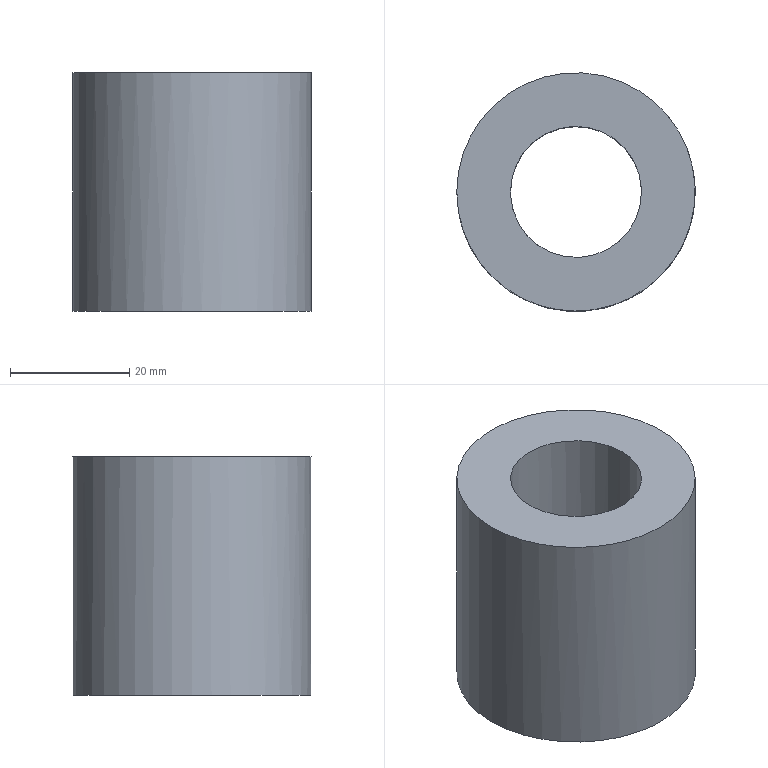Part | NX | features solid 2 | 1 solid | 4 faces | box 40 x 40 x 40 mm | volume 35060 mm3 | plane 2 | cylinder 2 | commonest cylinder face diameters 22 x1 40 x1
STEP:
#1=CARTESIAN_POINT('',(-644.963,510.927,170.));
#2=VERTEX_POINT('',#1);
#3=CARTESIAN_POINT('',(-643.053,521.759,170.));
#4=DIRECTION('',(0.,0.,-1.));
#5=DIRECTION('',(-0.1736,-0.9848,0.));
#6=AXIS2_PLACEMENT_3D('',#3,#4,#5);
#7=CIRCLE('',#6,11.);
#8=EDGE_CURVE('',#2,#2,#7,.T.);
#9=ORIENTED_EDGE('',*,*,#8,.T.);
#10=EDGE_LOOP('',(#9));
#11=FACE_BOUND('',#10,.T.);
#12=CARTESIAN_POINT('',(-646.526,502.063,170.));
#13=VERTEX_POINT('',#12);
#14=CARTESIAN_POINT('',(-643.053,521.759,170.));
#15=DIRECTION('',(0.,0.,-1.));
#16=DIRECTION('',(-0.1736,-0.9848,0.));
#17=AXIS2_PLACEMENT_3D('',#14,#15,#16);
#18=CIRCLE('',#17,20.);
#19=EDGE_CURVE('',#13,#13,#18,.T.);
#20=ORIENTED_EDGE('',*,*,#19,.F.);
#21=EDGE_LOOP('',(#20));
#22=FACE_BOUND('',#21,.T.);
#23=CARTESIAN_POINT('',(-643.053,521.759,170.));
#24=DIRECTION('',(0.,0.,1.));
#25=DIRECTION('',(0.1736,0.9848,0.));
#26=AXIS2_PLACEMENT_3D('',#23,#24,#25);
#27=PLANE('',#26);
#28=ADVANCED_FACE('',(#11,#22),#27,.T.);
#29=CARTESIAN_POINT('',(-654.053,521.759,130.));
#30=VERTEX_POINT('',#29);
#31=CARTESIAN_POINT('',(-643.053,521.759,130.));
#32=DIRECTION('',(0.,0.,-1.));
#33=DIRECTION('',(-1.,0.,0.));
#34=AXIS2_PLACEMENT_3D('',#31,#32,#33);
#35=CIRCLE('',#34,11.);
#36=EDGE_CURVE('',#30,#30,#35,.T.);
#37=ORIENTED_EDGE('',*,*,#36,.F.);
#38=EDGE_LOOP('',(#37));
#39=FACE_BOUND('',#38,.T.);
#40=CARTESIAN_POINT('',(-663.053,521.759,130.));
#41=VERTEX_POINT('',#40);
#42=CARTESIAN_POINT('',(-643.053,521.759,130.));
#43=DIRECTION('',(0.,0.,-1.));
#44=DIRECTION('',(-1.,0.,0.));
#45=AXIS2_PLACEMENT_3D('',#42,#43,#44);
#46=CIRCLE('',#45,20.);
#47=EDGE_CURVE('',#41,#41,#46,.F.);
#48=ORIENTED_EDGE('',*,*,#47,.F.);
#49=EDGE_LOOP('',(#48));
#50=FACE_BOUND('',#49,.T.);
#51=CARTESIAN_POINT('',(-643.053,521.759,130.));
#52=DIRECTION('',(0.,0.,-1.));
#53=DIRECTION('',(-0.1736,-0.9848,0.));
#54=AXIS2_PLACEMENT_3D('',#51,#52,#53);
#55=PLANE('',#54);
#56=ADVANCED_FACE('',(#39,#50),#55,.T.);
#57=ORIENTED_EDGE('',*,*,#19,.T.);
#58=EDGE_LOOP('',(#57));
#59=FACE_BOUND('',#58,.T.);
#60=ORIENTED_EDGE('',*,*,#47,.T.);
#61=EDGE_LOOP('',(#60));
#62=FACE_BOUND('',#61,.T.);
#63=CARTESIAN_POINT('',(-643.053,521.759,117.));
#64=DIRECTION('',(0.,0.,1.));
#65=DIRECTION('',(0.1736,0.9848,0.));
#66=AXIS2_PLACEMENT_3D('',#63,#64,#65);
#67=CYLINDRICAL_SURFACE('',#66,20.);
#68=ADVANCED_FACE('',(#59,#62),#67,.T.);
#69=ORIENTED_EDGE('',*,*,#36,.T.);
#70=EDGE_LOOP('',(#69));
#71=FACE_BOUND('',#70,.T.);
#72=ORIENTED_EDGE('',*,*,#8,.F.);
#73=EDGE_LOOP('',(#72));
#74=FACE_BOUND('',#73,.T.);
#75=CARTESIAN_POINT('',(-643.053,521.759,157.));
#76=DIRECTION('',(0.,0.,-1.));
#77=DIRECTION('',(-0.1736,-0.9848,0.));
#78=AXIS2_PLACEMENT_3D('',#75,#76,#77);
#79=CYLINDRICAL_SURFACE('',#78,11.);
#80=ADVANCED_FACE('',(#71,#74),#79,.F.);
#81=CLOSED_SHELL('',(#28,#56,#68,#80));
#82=MANIFOLD_SOLID_BREP('',#81);
#83=(LENGTH_UNIT()NAMED_UNIT(*)SI_UNIT(.MILLI.,.METRE.));
#84=UNCERTAINTY_MEASURE_WITH_UNIT(LENGTH_MEASURE(0.00001),#83,'','');
#85=(NAMED_UNIT(*)PLANE_ANGLE_UNIT()SI_UNIT($,.RADIAN.));
#86=(NAMED_UNIT(*)SI_UNIT($,.STERADIAN.)SOLID_ANGLE_UNIT());
#87=(GEOMETRIC_REPRESENTATION_CONTEXT(3)GLOBAL_UNCERTAINTY_ASSIGNED_CONTEXT((#84))GLOBAL_UNIT_ASSIGNED_CONTEXT((#83,#85,#86))REPRESENTATION_CONTEXT('',''));
#88=ADVANCED_BREP_SHAPE_REPRESENTATION('',(#82),#87);